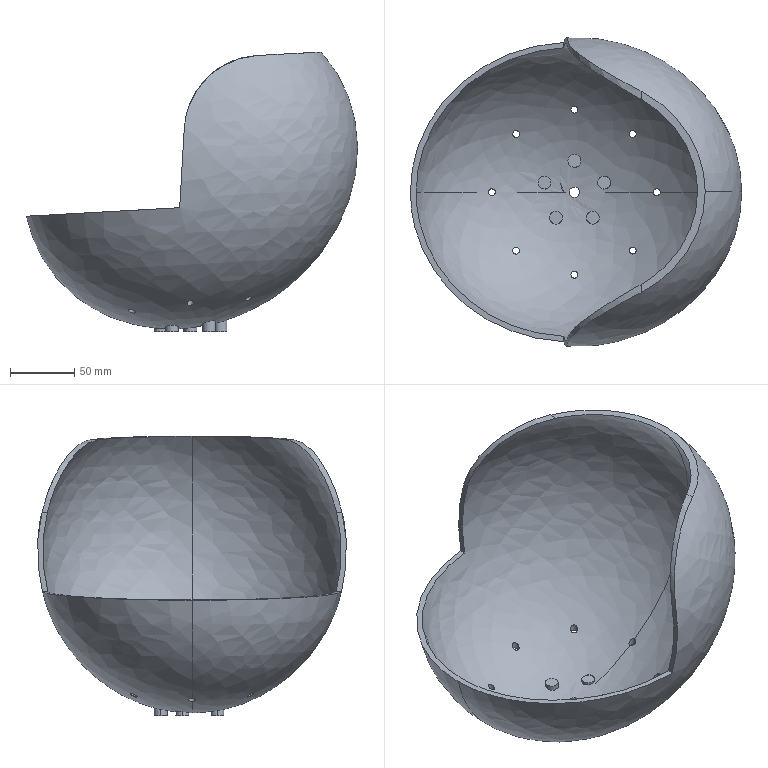Part | SolidWorks | features ICE 4, Bending 1, Fillet 1, Revolution 1, Shell 1 | 6 solids | 58 faces | box 256.913 x 240.018 x 217.091 mm | volume 479956 mm3 | cylinder 38 | plane 12 | spline 8 | commonest cylinder face diameters 10 x20 5.322 x16 8 x2